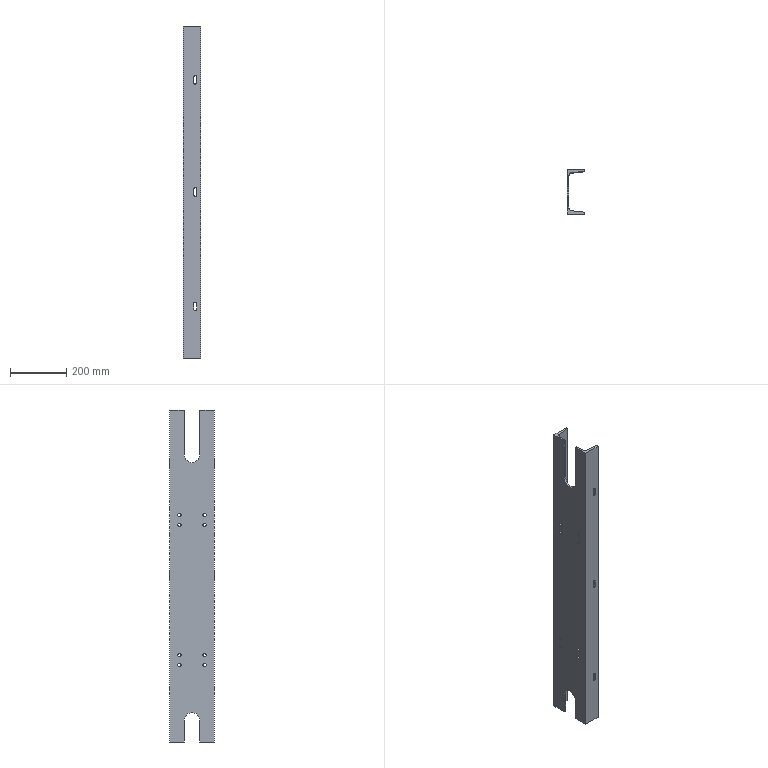Part | STEP file | Conveyor belt bracket | 1 solid | 69 faces | box 63 x 160 x 1184 mm | volume 2475798 mm3 | cylinder 41 | plane 28 | commonest cylinder face diameters 11 x18 12 x16 55 x3 10 x2 20 x2